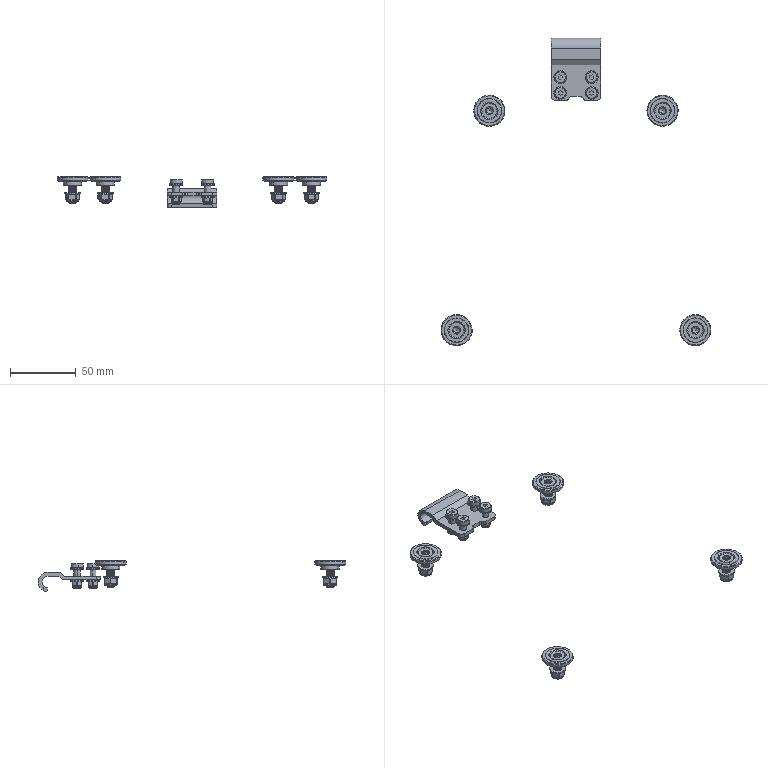Part | SolidWorks | 41 solids | 1579 faces | box 206.1 x 234.737 x 23.954 mm | volume 19949 mm3 | cylinder 569 | spline 356 | cone 272 | torus 192 | plane 182 | sphere 8 | commonest cylinder face diameters 6 x145 5 x71 1 x60 3.2 x39 1.01 x36 2.274 x32